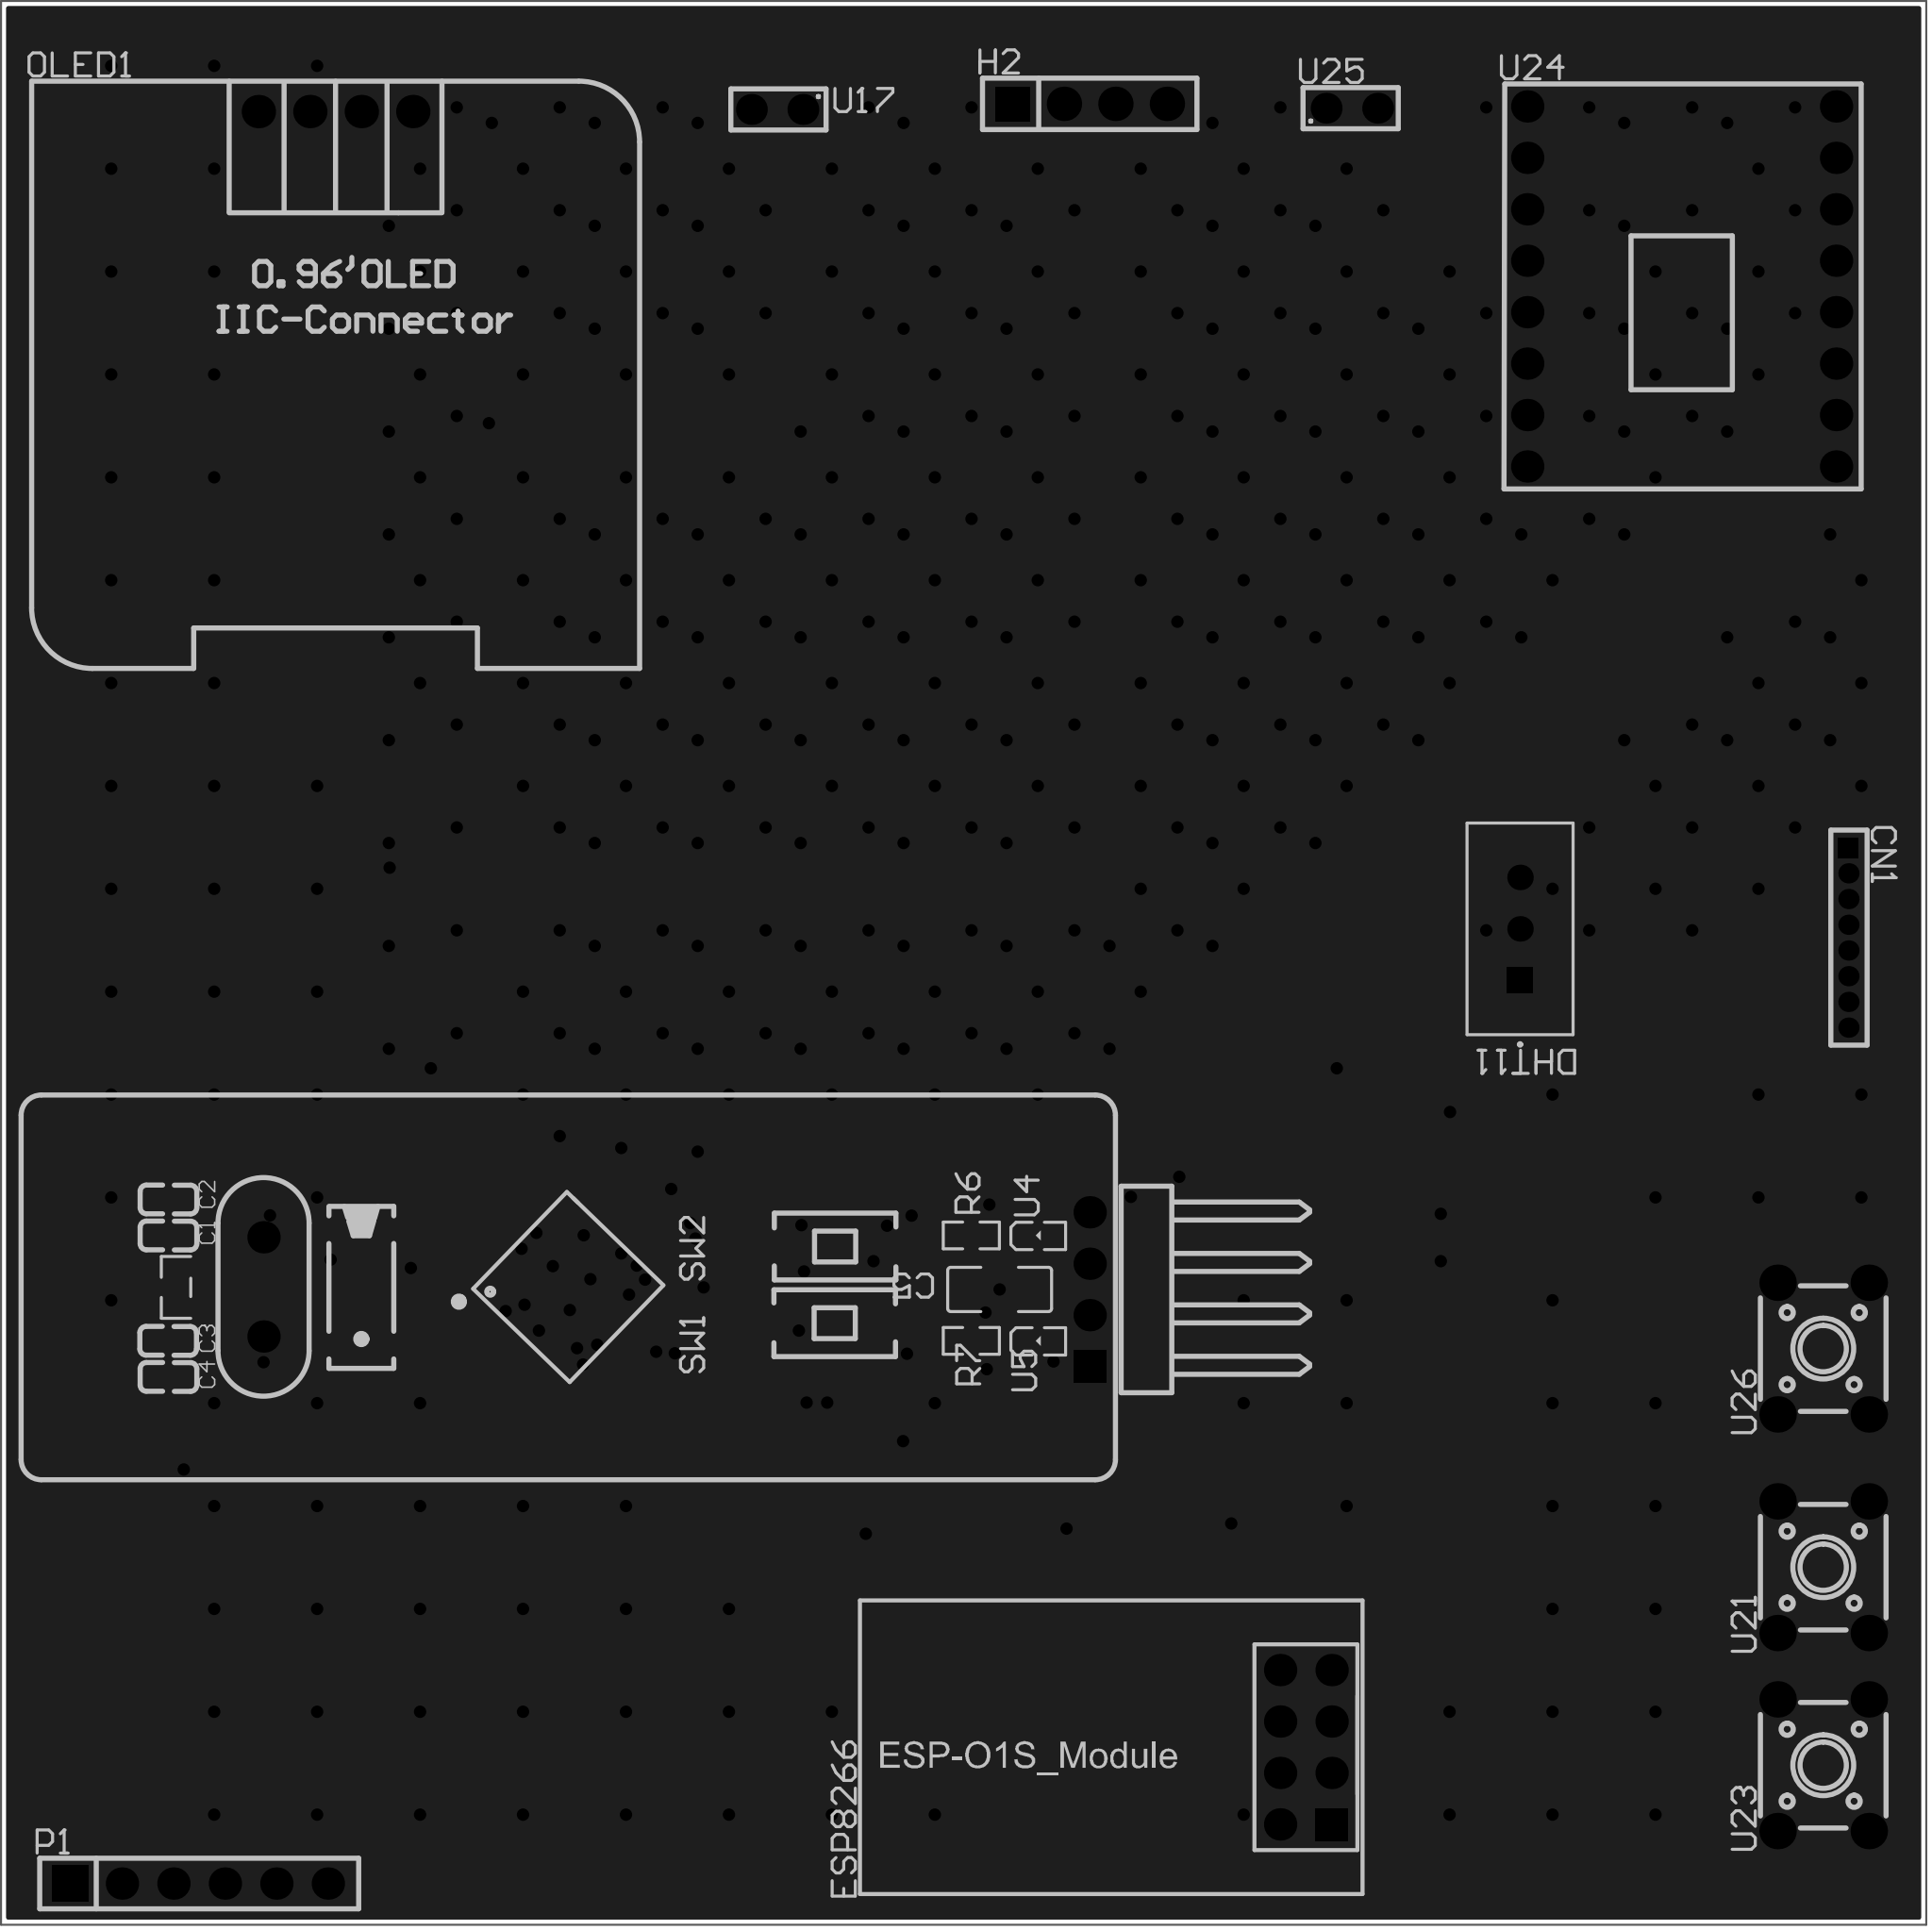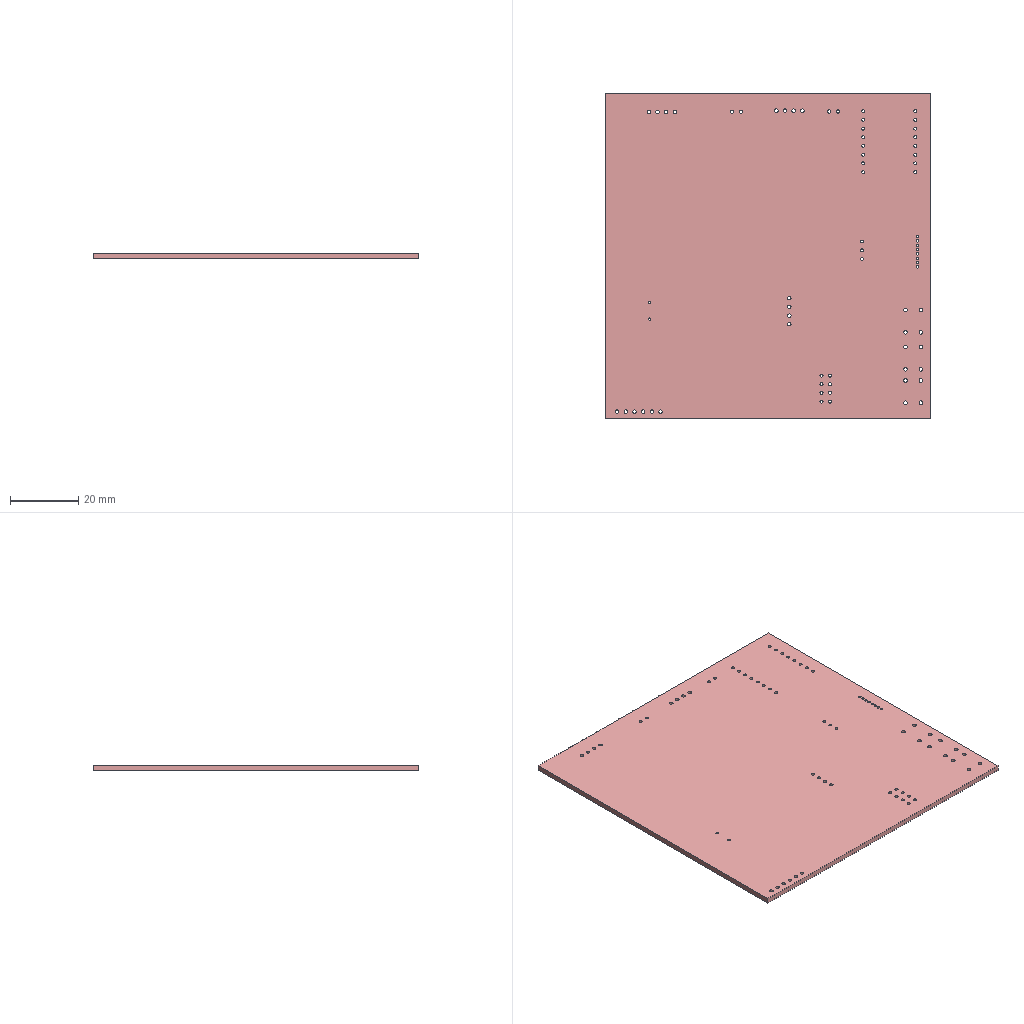Circuit board layout | Altium Designer | box 95 x 95 x 1.6 mm
Layer stack:
# Altium Designer layer stack of  (unit mm; dielectric type: 0 none, 1 core, 2 prepreg, 3 surface material)
index,name,kind,layer,copper_thickness_mm,dielectric_type,dielectric_thickness_mm,dielectric_material,dielectric_constant
0,Top Paste Mask Layer,other,,,,,,
1,Top Silkscreen Layer,other,,,,,,
2,Top Solder Mask Layer,dielectric,,,3,0.01,,3.3
3,Top Layer,copper,Top Layer,0.035,,,,
4,Dielectric1,dielectric,,,3,1.51,FR4,4.5
5,Bottom Layer,copper,Bottom Layer,0.035,,,,
6,Bottom Solder Mask Layer,dielectric,,,3,0.01,,3.3
7,Bottom Silkscreen Layer,other,,,,,,
8,Bottom Paste Mask Layer,other,,,,,,
# drill layer pairs: low layer,high layer
drill_pair,Top Layer,Bottom Layer
Part placement:
Designator,Comment,Layer,Footprint,Center-X(mm),Center-Y(mm),Rotation
CN1,2.0mm*8P female header,TopLayer,HDR-TH_8P-P1.27_2.0MM-8P,169.774,129.007,270
DHT11,,TopLayer,PIN3直插DHT11,153.569,129.439,180
ESP8266,,TopLayer,ESP8266-01S_Module,143.002,89.027,90
H2,4P,TopLayer,HDR-TH_4P-P2.54-V-M-3,132.334,170.18,0
OLED1,,TopLayer,0.96OLED_4P,95.123,169.799,0
P1,MINI USB power input module,TopLayer,HDR-TH_6P-P2.54-V-F,88.392,82.296,0
U17,,TopLayer,2p排针,116.912,169.905,180
U21,UP,TopLayer,KEY-TH_4P复位按键,168.529,97.917,90
U23,DOWN,TopLayer,KEY-TH_4P复位按键,168.529,88.138,90
U24,,TopLayer,TB6612电机驱动,161.544,161.163,0
U25,,TopLayer,2p排针,145.273,169.965,0
U26,UP,TopLayer,KEY-TH_4P复位按键,168.529,108.712,90
C4,10uF,TopLayer,C0603,86.883,107.31,0
U5,42-51/GHC-YW2X2K/3T,TopLayer,LED-SMD_L1.6-W0.8-FD_GREEN-1,129.794,109.093,180
R7,510Ω,TopLayer,R0603,126.492,109.093,180
C3,100nF,TopLayer,C0603,86.868,109.093,0
SW1,TS-1101-C-W,TopLayer,SW-SMD_L6.0-W3.3-LS8.0,119.888,109.985,0
C5,100uF,TopLayer,C1206,127.889,111.633,180
H1,A254AD-WD04P,TopLayer,HDR-TH_4P-P2.54-H-M-W10.2,132.334,111.633,90
U1,STM32F103C8T6,TopLayer,LQFP-48_L7.0-W7.0-P0.50-LS9.0-BL,106.604,111.735,316
LDO1,SC662K-3.3V,TopLayer,SOT-23-3_L2.9-W1.3-P1.90-LS2.4-BR,87.249,111.735,0
X2,32.768kHz,TopLayer,MC-306_4P-L8.0-W3.2-P5.5-BL,96.393,111.735,270
X1,8MHz,TopLayer,OSC-TH_L10.0-W4.5-P5.00,91.567,111.76,180
SW2,TS-1101-C-W,TopLayer,SW-SMD_L6.0-W3.3-LS8.0,119.634,113.735,180
U4,42-51/GHC-YW2X2K/3T,TopLayer,LED-SMD_L1.6-W0.8-FD_GREEN-1,129.794,114.3,180
C1,10uF,TopLayer,C0603,86.868,114.3,180
R6,510Ω,TopLayer,R0603,126.492,114.3,180
C2,100nF,TopLayer,C0603,86.868,116.078,180
C8,20pF,BottomLayer,C0603,90.805,106.934,0
R3,1kΩ,BottomLayer,R0603,129.794,107.061,0
R5,10kΩ,BottomLayer,R0603,124.333,107.188,180
C16,4.7nF,BottomLayer,C0603,120.753,108.458,180
C11,100nF,BottomLayer,C0603,116.332,108.458,180
C9,20pF,BottomLayer,C0603,94.742,111.633,90
C10,20pF,BottomLayer,C0603,98.044,111.735,90
C15,100nF,BottomLayer,C0603,120.777,111.735,180
C12,100nF,BottomLayer,C0603,116.332,111.735,180
C13,100nF,BottomLayer,C0603,116.332,114.935,180
C14,100nF,BottomLayer,C0603,120.777,115.062,180
C7,20pF,BottomLayer,C0603,90.932,116.205,0
R4,10kΩ,BottomLayer,R0603,124.35,116.205,180
C6,100nF,BottomLayer,C0603,129.788,116.332,0
Pad and via stacks:
# Altium Designer via and pad stacks of  (unit mm). Each distinct definition once, with the count of objects using it.
# via: kind,start_layer,end_layer,hole_mm,diameter_mm,mode(0 simple;1 top-mid-bottom;2 full stack),diameter_per_layer,count,example_net
# pad: kind,layer,hole_mm,hole_type(0 round;1 square;2 slot),plating,top_size,top_shape(1 round;2 rect;3 octagon;9 rounded rect),mid_size,bottom_size,mode,footprint,size_per_layer,count,example
pad,Multi-Layer,0.7,0,plated,1x1,1,1x1,1x1,0,HDR-TH_8P-P1.27_2.0MM-8P,,7,CN1.7
pad,Multi-Layer,0.7,0,plated,1x1,2,1x1,1x1,0,HDR-TH_8P-P1.27_2.0MM-8P,,1,CN1.1
pad,Multi-Layer,0.84,0,plated,1.26x1.26,2,1.26x1.26,1.26x1.26,0,PIN3\u00D6\u00B1\u00B2\u00E5DHT11,,1,DHT11.1
pad,Multi-Layer,0.84,0,plated,1.26x1.26,1,1.26x1.26,1.26x1.26,0,PIN3\u00D6\u00B1\u00B2\u00E5DHT11,,2,DHT11.2
pad,Multi-Layer,0.9,0,plated,1.6x1.6,1,1.6x1.6,1.6x1.6,0,ESP8266-01S_Module,,7,ESP8266.7
pad,Multi-Layer,0.9,0,plated,1.6x1.6,2,1.6x1.6,1.6x1.6,0,ESP8266-01S_Module,,1,ESP8266.1
pad,Multi-Layer,1.1,0,plated,1.699x1.699,1,1.699x1.699,1.699x1.699,0,HDR-TH_4P-P2.54-V-M-3,,3,H2.4
pad,Multi-Layer,1.1,0,plated,1.699x1.699,2,1.699x1.699,1.699x1.699,0,HDR-TH_4P-P2.54-V-M-3,,1,H2.1
pad,Multi-Layer,1,0,plated,1.65x1.65,1,1.65x1.65,1.65x1.65,0,0.96OLED_4P,,4,OLED1.4
pad,Multi-Layer,1.02,0,plated,1.6x1.6,1,1.6x1.6,1.6x1.6,0,HDR-TH_6P-P2.54-V-F,,5,P1.6
pad,Multi-Layer,1.02,0,plated,1.8x1.8,2,1.8x1.8,1.8x1.8,0,HDR-TH_6P-P2.54-V-F,,1,P1.1
pad,Multi-Layer,0.9144,0,plated,1.524x1.524,1,1.524x1.524,1.524x1.524,0,2p\u00C5\u00C5\u00D5\u00EB,,4,U17.1
pad,Multi-Layer,1.1,2,plated,1.8x1.8,1,1.8x1.8,1.8x1.8,0,KEY-TH_4P\u00B8\u00B4\u00CE\u00BB\u00B0\u00B4\u00BC\u00FC,,12,U21.1
pad,Multi-Layer,0.9,0,plated,1.6x1.6,1,1.6x1.6,1.6x1.6,0,TB6612\u00B5\u00E7\u00BB\u00FA\u00C7\u00FD\u00B6\u00AF,,16,U24.1
pad,Multi-Layer,1,0,plated,1.6x1.6,1,1.6x1.6,1.6x1.6,0,HDR-TH_4P-P2.54-H-M-W10.2,,3,H1.4
pad,Multi-Layer,1,0,plated,1.6x1.6,2,1.6x1.6,1.6x1.6,0,HDR-TH_4P-P2.54-H-M-W10.2,,1,H1.1
pad,Multi-Layer,0.7,0,plated,1.6x1.6,1,1.6x1.6,1.6x1.6,0,OSC-TH_L10.0-W4.5-P5.00,,2,X1.2
pad,Top Layer,0,0,plated,0.8x0.9,2,0.8x0.9,0.8x0.9,0,C0603,,8,C4.2
pad,Top Layer,0,0,plated,0.8x0.7,2,0.8x0.7,0.8x0.7,0,LED-SMD_L1.6-W0.8-FD_GREEN-1,,4,U5.1
pad,Top Layer,0,0,plated,0.8065x0.864,2,0.8065x0.864,0.8065x0.864,0,R0603,,4,R7.2
pad,Top Layer,0,0,plated,1.9x1.5,2,1.9x1.5,1.9x1.5,0,SW-SMD_L6.0-W3.3-LS8.0,,4,SW1.1
pad,Top Layer,0,0,plated,1.485x1.728,2,1.485x1.728,1.485x1.728,0,C1206,,2,C5.2
pad,Top Layer,0,0,plated,0.27x1.5,1,0.27x1.5,0.27x1.5,0,LQFP-48_L7.0-W7.0-P0.50-LS9.0-BL,,24,U1.1
pad,Top Layer,0,0,plated,1.5x0.27,1,1.5x0.27,1.5x0.27,0,LQFP-48_L7.0-W7.0-P0.50-LS9.0-BL,,24,U1.13
pad,Top Layer,0,0,plated,1.25x0.7,2,1.25x0.7,1.25x0.7,0,SOT-23-3_L2.9-W1.3-P1.90-LS2.4-BR,,3,LDO1.1
pad,Top Layer,0,0,plated,0.9x1.3,2,0.9x1.3,0.9x1.3,0,MC-306_4P-L8.0-W3.2-P5.5-BL,,4,X2.1
pad,Bottom Layer,0,0,plated,0.8x0.9,2,0.8x0.9,0.8x0.9,0,C0603,,22,C8.2
pad,Bottom Layer,0,0,plated,0.8065x0.864,2,0.8065x0.864,0.8065x0.864,0,R0603,,6,R3.2
via,Top Layer,Bottom Layer,0.3048,0.61,0,,453,+5V
Copper pours:
name,layer,net,type(0 solid;1 hatched;2 none)
Top Layer-GND,Top Layer,GND,0
Bottom Layer-GND,Bottom Layer,GND,0
Design rules, without the lines most boards share:
# Altium Designer design rules of  (exported by Altium Designer, unit mm)
# columns: name | kind | enabled | priority | scope1 | scope2 | descriptor | typed fields (field=value)
copperThickness2oz | 0 | enabled | 1 | (InNet('+5V')) | All | Clearance Constraint (Gap=5.984mil) ((InNet('+5V'))),(All) | gap=0.152
copperThickness2oz_1 | 63 | enabled | 1 | All | All | Board Clearance Constraint (Gap=0mil) (All) |
copperThickness2oz_2 | 2 | enabled | 1 | (InNet('+5V')) | All | Width Constraint (Min=15mil) (Max=100mil) (Preferred=15mil) ((InNet('+5V'))) |
viaSize | 11 | enabled | 1 | All | All | Routing Via (MinHoleWidth=11.811mil) (MaxHoleWidth=248.032mil) (PreferredHoleWidth=12.008mil) (MinWidth=19.685mil) (MaxWidth=393.701mil) (PreferedWidth=24.016mil) (All) | via_min_hole=0.3 via_max_hole=6.3 via_preferred_diameter=0.61 via_preferred_hole=0.305
solderMaskExpansion | 13 | enabled | 2 | All | All | Solder Mask Expansion (Expansion =2.008mil) (All) | expansion=0.051